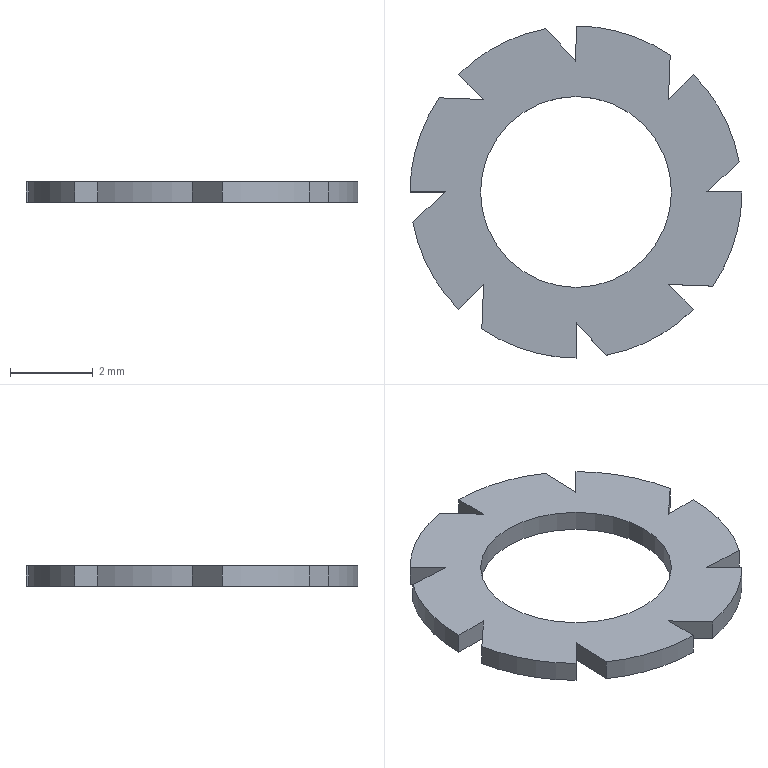Part | NX | features BREP 1 | 1 solid | 27 faces | box 8 x 8 x 0.5 mm | volume 15.56 mm3 | plane 18 | cylinder 9 | commonest cylinder face diameters 8 x8 4.6 x1
STEP:
#1=CARTESIAN_POINT('',(2.3,0.,0.));
#2=VERTEX_POINT('',#1);
#3=CARTESIAN_POINT('',(0.,0.,0.));
#4=DIRECTION('',(0.,0.,1.));
#5=DIRECTION('',(1.,0.,0.));
#6=AXIS2_PLACEMENT_3D('',#3,#4,#5);
#7=CIRCLE('',#6,2.3);
#8=EDGE_CURVE('',#2,#2,#7,.T.);
#9=ORIENTED_EDGE('',*,*,#8,.T.);
#10=EDGE_LOOP('',(#9));
#11=FACE_BOUND('',#10,.T.);
#12=CARTESIAN_POINT('',(2.3,0.,-0.5));
#13=VERTEX_POINT('',#12);
#14=CARTESIAN_POINT('',(0.,0.,-0.5));
#15=DIRECTION('',(0.,0.,1.));
#16=DIRECTION('',(1.,0.,0.));
#17=AXIS2_PLACEMENT_3D('',#14,#15,#16);
#18=CIRCLE('',#17,2.3);
#19=EDGE_CURVE('',#13,#13,#18,.T.);
#20=ORIENTED_EDGE('',*,*,#19,.F.);
#21=EDGE_LOOP('',(#20));
#22=FACE_BOUND('',#21,.T.);
#23=CARTESIAN_POINT('',(0.,0.,-0.5));
#24=DIRECTION('',(0.,0.,1.));
#25=DIRECTION('',(1.,0.,0.));
#26=AXIS2_PLACEMENT_3D('',#23,#24,#25);
#27=CYLINDRICAL_SURFACE('',#26,2.3);
#28=ADVANCED_FACE('',(#11,#22),#27,.F.);
#29=CARTESIAN_POINT('',(2.828,2.828,-0.5));
#30=VERTEX_POINT('',#29);
#31=CARTESIAN_POINT('',(2.828,2.828,0.));
#32=VERTEX_POINT('',#31);
#33=CARTESIAN_POINT('',(2.828,2.828,-0.5));
#34=DIRECTION('',(0.,0.,1.));
#35=VECTOR('',#34,1000.);
#36=LINE('',#33,#35);
#37=EDGE_CURVE('',#30,#32,#36,.T.);
#38=ORIENTED_EDGE('',*,*,#37,.T.);
#39=CARTESIAN_POINT('',(3.934,0.7243,0.));
#40=VERTEX_POINT('',#39);
#41=CARTESIAN_POINT('',(0.,0.,0.));
#42=DIRECTION('',(0.,0.,1.));
#43=DIRECTION('',(1.,0.,0.));
#44=AXIS2_PLACEMENT_3D('',#41,#42,#43);
#45=CIRCLE('',#44,4.);
#46=EDGE_CURVE('',#40,#32,#45,.T.);
#47=ORIENTED_EDGE('',*,*,#46,.F.);
#48=CARTESIAN_POINT('',(3.934,0.7243,-0.5));
#49=VERTEX_POINT('',#48);
#50=CARTESIAN_POINT('',(3.934,0.7243,-0.5));
#51=DIRECTION('',(0.,0.,1.));
#52=VECTOR('',#51,1000.);
#53=LINE('',#50,#52);
#54=EDGE_CURVE('',#49,#40,#53,.T.);
#55=ORIENTED_EDGE('',*,*,#54,.F.);
#56=CARTESIAN_POINT('',(0.,0.,-0.5));
#57=DIRECTION('',(0.,0.,1.));
#58=DIRECTION('',(1.,0.,0.));
#59=AXIS2_PLACEMENT_3D('',#56,#57,#58);
#60=CIRCLE('',#59,4.);
#61=EDGE_CURVE('',#49,#30,#60,.T.);
#62=ORIENTED_EDGE('',*,*,#61,.T.);
#63=EDGE_LOOP('',(#38,#47,#55,#62));
#64=FACE_BOUND('',#63,.T.);
#65=CARTESIAN_POINT('',(0.,0.,-0.5));
#66=DIRECTION('',(0.,0.,1.));
#67=DIRECTION('',(1.,0.,0.));
#68=AXIS2_PLACEMENT_3D('',#65,#66,#67);
#69=CYLINDRICAL_SURFACE('',#68,4.);
#70=ADVANCED_FACE('',(#64),#69,.T.);
#71=CARTESIAN_POINT('',(4.,0.,-0.5));
#72=VERTEX_POINT('',#71);
#73=CARTESIAN_POINT('',(4.,0.,0.));
#74=VERTEX_POINT('',#73);
#75=CARTESIAN_POINT('',(4.,0.,-0.5));
#76=DIRECTION('',(0.,0.,1.));
#77=VECTOR('',#76,1000.);
#78=LINE('',#75,#77);
#79=EDGE_CURVE('',#72,#74,#78,.T.);
#80=ORIENTED_EDGE('',*,*,#79,.T.);
#81=CARTESIAN_POINT('',(3.294,-2.27,0.));
#82=VERTEX_POINT('',#81);
#83=CARTESIAN_POINT('',(0.,0.,0.));
#84=DIRECTION('',(0.,0.,1.));
#85=DIRECTION('',(1.,0.,0.));
#86=AXIS2_PLACEMENT_3D('',#83,#84,#85);
#87=CIRCLE('',#86,4.);
#88=EDGE_CURVE('',#82,#74,#87,.T.);
#89=ORIENTED_EDGE('',*,*,#88,.F.);
#90=CARTESIAN_POINT('',(3.294,-2.27,-0.5));
#91=VERTEX_POINT('',#90);
#92=CARTESIAN_POINT('',(3.294,-2.27,-0.5));
#93=DIRECTION('',(0.,0.,1.));
#94=VECTOR('',#93,1000.);
#95=LINE('',#92,#94);
#96=EDGE_CURVE('',#91,#82,#95,.T.);
#97=ORIENTED_EDGE('',*,*,#96,.F.);
#98=CARTESIAN_POINT('',(0.,0.,-0.5));
#99=DIRECTION('',(0.,0.,1.));
#100=DIRECTION('',(1.,0.,0.));
#101=AXIS2_PLACEMENT_3D('',#98,#99,#100);
#102=CIRCLE('',#101,4.);
#103=EDGE_CURVE('',#91,#72,#102,.T.);
#104=ORIENTED_EDGE('',*,*,#103,.T.);
#105=EDGE_LOOP('',(#80,#89,#97,#104));
#106=FACE_BOUND('',#105,.T.);
#107=CARTESIAN_POINT('',(0.,0.,-0.5));
#108=DIRECTION('',(0.,0.,1.));
#109=DIRECTION('',(1.,0.,0.));
#110=AXIS2_PLACEMENT_3D('',#107,#108,#109);
#111=CYLINDRICAL_SURFACE('',#110,4.);
#112=ADVANCED_FACE('',(#106),#111,.T.);
#113=CARTESIAN_POINT('',(2.828,-2.828,-0.5));
#114=VERTEX_POINT('',#113);
#115=CARTESIAN_POINT('',(2.828,-2.828,0.));
#116=VERTEX_POINT('',#115);
#117=CARTESIAN_POINT('',(2.828,-2.828,-0.5));
#118=DIRECTION('',(0.,0.,1.));
#119=VECTOR('',#118,1000.);
#120=LINE('',#117,#119);
#121=EDGE_CURVE('',#114,#116,#120,.T.);
#122=ORIENTED_EDGE('',*,*,#121,.T.);
#123=CARTESIAN_POINT('',(0.7243,-3.934,0.));
#124=VERTEX_POINT('',#123);
#125=CARTESIAN_POINT('',(0.,0.,0.));
#126=DIRECTION('',(0.,0.,1.));
#127=DIRECTION('',(1.,0.,0.));
#128=AXIS2_PLACEMENT_3D('',#125,#126,#127);
#129=CIRCLE('',#128,4.);
#130=EDGE_CURVE('',#124,#116,#129,.T.);
#131=ORIENTED_EDGE('',*,*,#130,.F.);
#132=CARTESIAN_POINT('',(0.7243,-3.934,-0.5));
#133=VERTEX_POINT('',#132);
#134=CARTESIAN_POINT('',(0.7243,-3.934,-0.5));
#135=DIRECTION('',(0.,0.,1.));
#136=VECTOR('',#135,1000.);
#137=LINE('',#134,#136);
#138=EDGE_CURVE('',#133,#124,#137,.T.);
#139=ORIENTED_EDGE('',*,*,#138,.F.);
#140=CARTESIAN_POINT('',(0.,0.,-0.5));
#141=DIRECTION('',(0.,0.,1.));
#142=DIRECTION('',(1.,0.,0.));
#143=AXIS2_PLACEMENT_3D('',#140,#141,#142);
#144=CIRCLE('',#143,4.);
#145=EDGE_CURVE('',#133,#114,#144,.T.);
#146=ORIENTED_EDGE('',*,*,#145,.T.);
#147=EDGE_LOOP('',(#122,#131,#139,#146));
#148=FACE_BOUND('',#147,.T.);
#149=CARTESIAN_POINT('',(0.,0.,-0.5));
#150=DIRECTION('',(0.,0.,1.));
#151=DIRECTION('',(1.,0.,0.));
#152=AXIS2_PLACEMENT_3D('',#149,#150,#151);
#153=CYLINDRICAL_SURFACE('',#152,4.);
#154=ADVANCED_FACE('',(#148),#153,.T.);
#155=CARTESIAN_POINT('',(0.,-4.,-0.5));
#156=VERTEX_POINT('',#155);
#157=CARTESIAN_POINT('',(0.,-4.,0.));
#158=VERTEX_POINT('',#157);
#159=CARTESIAN_POINT('',(0.,-4.,-0.5));
#160=DIRECTION('',(0.,0.,1.));
#161=VECTOR('',#160,1000.);
#162=LINE('',#159,#161);
#163=EDGE_CURVE('',#156,#158,#162,.T.);
#164=ORIENTED_EDGE('',*,*,#163,.T.);
#165=CARTESIAN_POINT('',(-2.27,-3.294,0.));
#166=VERTEX_POINT('',#165);
#167=CARTESIAN_POINT('',(0.,0.,0.));
#168=DIRECTION('',(0.,0.,1.));
#169=DIRECTION('',(1.,0.,0.));
#170=AXIS2_PLACEMENT_3D('',#167,#168,#169);
#171=CIRCLE('',#170,4.);
#172=EDGE_CURVE('',#166,#158,#171,.T.);
#173=ORIENTED_EDGE('',*,*,#172,.F.);
#174=CARTESIAN_POINT('',(-2.27,-3.294,-0.5));
#175=VERTEX_POINT('',#174);
#176=CARTESIAN_POINT('',(-2.27,-3.294,-0.5));
#177=DIRECTION('',(0.,0.,1.));
#178=VECTOR('',#177,1000.);
#179=LINE('',#176,#178);
#180=EDGE_CURVE('',#175,#166,#179,.T.);
#181=ORIENTED_EDGE('',*,*,#180,.F.);
#182=CARTESIAN_POINT('',(0.,0.,-0.5));
#183=DIRECTION('',(0.,0.,1.));
#184=DIRECTION('',(1.,0.,0.));
#185=AXIS2_PLACEMENT_3D('',#182,#183,#184);
#186=CIRCLE('',#185,4.);
#187=EDGE_CURVE('',#175,#156,#186,.T.);
#188=ORIENTED_EDGE('',*,*,#187,.T.);
#189=EDGE_LOOP('',(#164,#173,#181,#188));
#190=FACE_BOUND('',#189,.T.);
#191=CARTESIAN_POINT('',(0.,0.,-0.5));
#192=DIRECTION('',(0.,0.,1.));
#193=DIRECTION('',(1.,0.,0.));
#194=AXIS2_PLACEMENT_3D('',#191,#192,#193);
#195=CYLINDRICAL_SURFACE('',#194,4.);
#196=ADVANCED_FACE('',(#190),#195,.T.);
#197=CARTESIAN_POINT('',(-2.828,-2.828,-0.5));
#198=VERTEX_POINT('',#197);
#199=CARTESIAN_POINT('',(-2.828,-2.828,0.));
#200=VERTEX_POINT('',#199);
#201=CARTESIAN_POINT('',(-2.828,-2.828,-0.5));
#202=DIRECTION('',(0.,0.,1.));
#203=VECTOR('',#202,1000.);
#204=LINE('',#201,#203);
#205=EDGE_CURVE('',#198,#200,#204,.T.);
#206=ORIENTED_EDGE('',*,*,#205,.T.);
#207=CARTESIAN_POINT('',(-3.934,-0.7243,0.));
#208=VERTEX_POINT('',#207);
#209=CARTESIAN_POINT('',(0.,0.,0.));
#210=DIRECTION('',(0.,0.,1.));
#211=DIRECTION('',(1.,0.,0.));
#212=AXIS2_PLACEMENT_3D('',#209,#210,#211);
#213=CIRCLE('',#212,4.);
#214=EDGE_CURVE('',#208,#200,#213,.T.);
#215=ORIENTED_EDGE('',*,*,#214,.F.);
#216=CARTESIAN_POINT('',(-3.934,-0.7243,-0.5));
#217=VERTEX_POINT('',#216);
#218=CARTESIAN_POINT('',(-3.934,-0.7243,-0.5));
#219=DIRECTION('',(0.,0.,1.));
#220=VECTOR('',#219,1000.);
#221=LINE('',#218,#220);
#222=EDGE_CURVE('',#217,#208,#221,.T.);
#223=ORIENTED_EDGE('',*,*,#222,.F.);
#224=CARTESIAN_POINT('',(0.,0.,-0.5));
#225=DIRECTION('',(0.,0.,1.));
#226=DIRECTION('',(1.,0.,0.));
#227=AXIS2_PLACEMENT_3D('',#224,#225,#226);
#228=CIRCLE('',#227,4.);
#229=EDGE_CURVE('',#217,#198,#228,.T.);
#230=ORIENTED_EDGE('',*,*,#229,.T.);
#231=EDGE_LOOP('',(#206,#215,#223,#230));
#232=FACE_BOUND('',#231,.T.);
#233=CARTESIAN_POINT('',(0.,0.,-0.5));
#234=DIRECTION('',(0.,0.,1.));
#235=DIRECTION('',(1.,0.,0.));
#236=AXIS2_PLACEMENT_3D('',#233,#234,#235);
#237=CYLINDRICAL_SURFACE('',#236,4.);
#238=ADVANCED_FACE('',(#232),#237,.T.);
#239=CARTESIAN_POINT('',(-4.,0.,-0.5));
#240=VERTEX_POINT('',#239);
#241=CARTESIAN_POINT('',(-4.,0.,0.));
#242=VERTEX_POINT('',#241);
#243=CARTESIAN_POINT('',(-4.,0.,-0.5));
#244=DIRECTION('',(0.,0.,1.));
#245=VECTOR('',#244,1000.);
#246=LINE('',#243,#245);
#247=EDGE_CURVE('',#240,#242,#246,.T.);
#248=ORIENTED_EDGE('',*,*,#247,.T.);
#249=CARTESIAN_POINT('',(-3.294,2.27,0.));
#250=VERTEX_POINT('',#249);
#251=CARTESIAN_POINT('',(0.,0.,0.));
#252=DIRECTION('',(0.,0.,1.));
#253=DIRECTION('',(1.,0.,0.));
#254=AXIS2_PLACEMENT_3D('',#251,#252,#253);
#255=CIRCLE('',#254,4.);
#256=EDGE_CURVE('',#250,#242,#255,.T.);
#257=ORIENTED_EDGE('',*,*,#256,.F.);
#258=CARTESIAN_POINT('',(-3.294,2.27,-0.5));
#259=VERTEX_POINT('',#258);
#260=CARTESIAN_POINT('',(-3.294,2.27,-0.5));
#261=DIRECTION('',(0.,0.,1.));
#262=VECTOR('',#261,1000.);
#263=LINE('',#260,#262);
#264=EDGE_CURVE('',#259,#250,#263,.T.);
#265=ORIENTED_EDGE('',*,*,#264,.F.);
#266=CARTESIAN_POINT('',(0.,0.,-0.5));
#267=DIRECTION('',(0.,0.,1.));
#268=DIRECTION('',(1.,0.,0.));
#269=AXIS2_PLACEMENT_3D('',#266,#267,#268);
#270=CIRCLE('',#269,4.);
#271=EDGE_CURVE('',#259,#240,#270,.T.);
#272=ORIENTED_EDGE('',*,*,#271,.T.);
#273=EDGE_LOOP('',(#248,#257,#265,#272));
#274=FACE_BOUND('',#273,.T.);
#275=CARTESIAN_POINT('',(0.,0.,-0.5));
#276=DIRECTION('',(0.,0.,1.));
#277=DIRECTION('',(1.,0.,0.));
#278=AXIS2_PLACEMENT_3D('',#275,#276,#277);
#279=CYLINDRICAL_SURFACE('',#278,4.);
#280=ADVANCED_FACE('',(#274),#279,.T.);
#281=CARTESIAN_POINT('',(-2.828,2.828,-0.5));
#282=VERTEX_POINT('',#281);
#283=CARTESIAN_POINT('',(-2.828,2.828,0.));
#284=VERTEX_POINT('',#283);
#285=CARTESIAN_POINT('',(-2.828,2.828,-0.5));
#286=DIRECTION('',(0.,0.,1.));
#287=VECTOR('',#286,1000.);
#288=LINE('',#285,#287);
#289=EDGE_CURVE('',#282,#284,#288,.T.);
#290=ORIENTED_EDGE('',*,*,#289,.T.);
#291=CARTESIAN_POINT('',(-0.7243,3.934,0.));
#292=VERTEX_POINT('',#291);
#293=CARTESIAN_POINT('',(0.,0.,0.));
#294=DIRECTION('',(0.,0.,1.));
#295=DIRECTION('',(1.,0.,0.));
#296=AXIS2_PLACEMENT_3D('',#293,#294,#295);
#297=CIRCLE('',#296,4.);
#298=EDGE_CURVE('',#292,#284,#297,.T.);
#299=ORIENTED_EDGE('',*,*,#298,.F.);
#300=CARTESIAN_POINT('',(-0.7243,3.934,-0.5));
#301=VERTEX_POINT('',#300);
#302=CARTESIAN_POINT('',(-0.7243,3.934,-0.5));
#303=DIRECTION('',(0.,0.,1.));
#304=VECTOR('',#303,1000.);
#305=LINE('',#302,#304);
#306=EDGE_CURVE('',#301,#292,#305,.T.);
#307=ORIENTED_EDGE('',*,*,#306,.F.);
#308=CARTESIAN_POINT('',(0.,0.,-0.5));
#309=DIRECTION('',(0.,0.,1.));
#310=DIRECTION('',(1.,0.,0.));
#311=AXIS2_PLACEMENT_3D('',#308,#309,#310);
#312=CIRCLE('',#311,4.);
#313=EDGE_CURVE('',#301,#282,#312,.T.);
#314=ORIENTED_EDGE('',*,*,#313,.T.);
#315=EDGE_LOOP('',(#290,#299,#307,#314));
#316=FACE_BOUND('',#315,.T.);
#317=CARTESIAN_POINT('',(0.,0.,-0.5));
#318=DIRECTION('',(0.,0.,1.));
#319=DIRECTION('',(1.,0.,0.));
#320=AXIS2_PLACEMENT_3D('',#317,#318,#319);
#321=CYLINDRICAL_SURFACE('',#320,4.);
#322=ADVANCED_FACE('',(#316),#321,.T.);
#323=CARTESIAN_POINT('',(2.27,3.294,-0.5));
#324=VERTEX_POINT('',#323);
#325=CARTESIAN_POINT('',(2.27,3.294,0.));
#326=VERTEX_POINT('',#325);
#327=CARTESIAN_POINT('',(2.27,3.294,-0.5));
#328=DIRECTION('',(0.,0.,1.));
#329=VECTOR('',#328,1000.);
#330=LINE('',#327,#329);
#331=EDGE_CURVE('',#324,#326,#330,.T.);
#332=ORIENTED_EDGE('',*,*,#331,.F.);
#333=CARTESIAN_POINT('',(0.,4.,-0.5));
#334=VERTEX_POINT('',#333);
#335=CARTESIAN_POINT('',(0.,0.,-0.5));
#336=DIRECTION('',(0.,0.,1.));
#337=DIRECTION('',(1.,0.,0.));
#338=AXIS2_PLACEMENT_3D('',#335,#336,#337);
#339=CIRCLE('',#338,4.);
#340=EDGE_CURVE('',#324,#334,#339,.T.);
#341=ORIENTED_EDGE('',*,*,#340,.T.);
#342=CARTESIAN_POINT('',(0.,4.,0.));
#343=VERTEX_POINT('',#342);
#344=CARTESIAN_POINT('',(0.,4.,-0.5));
#345=DIRECTION('',(0.,0.,1.));
#346=VECTOR('',#345,1000.);
#347=LINE('',#344,#346);
#348=EDGE_CURVE('',#334,#343,#347,.T.);
#349=ORIENTED_EDGE('',*,*,#348,.T.);
#350=CARTESIAN_POINT('',(0.,0.,0.));
#351=DIRECTION('',(0.,0.,1.));
#352=DIRECTION('',(1.,0.,0.));
#353=AXIS2_PLACEMENT_3D('',#350,#351,#352);
#354=CIRCLE('',#353,4.);
#355=EDGE_CURVE('',#326,#343,#354,.T.);
#356=ORIENTED_EDGE('',*,*,#355,.F.);
#357=EDGE_LOOP('',(#332,#341,#349,#356));
#358=FACE_BOUND('',#357,.T.);
#359=CARTESIAN_POINT('',(0.,0.,-0.5));
#360=DIRECTION('',(0.,0.,1.));
#361=DIRECTION('',(1.,0.,0.));
#362=AXIS2_PLACEMENT_3D('',#359,#360,#361);
#363=CYLINDRICAL_SURFACE('',#362,4.);
#364=ADVANCED_FACE('',(#358),#363,.T.);
#365=ORIENTED_EDGE('',*,*,#19,.T.);
#366=EDGE_LOOP('',(#365));
#367=FACE_BOUND('',#366,.T.);
#368=CARTESIAN_POINT('',(2.227,2.227,-0.5));
#369=VERTEX_POINT('',#368);
#370=CARTESIAN_POINT('',(2.227,2.227,-0.5));
#371=DIRECTION('',(-0.03947,-0.9992,0.));
#372=VECTOR('',#371,1000.);
#373=LINE('',#370,#372);
#374=EDGE_CURVE('',#324,#369,#373,.T.);
#375=ORIENTED_EDGE('',*,*,#374,.T.);
#376=CARTESIAN_POINT('',(2.828,2.828,-0.5));
#377=DIRECTION('',(0.7071,0.7071,0.));
#378=VECTOR('',#377,1000.);
#379=LINE('',#376,#378);
#380=EDGE_CURVE('',#369,#30,#379,.T.);
#381=ORIENTED_EDGE('',*,*,#380,.T.);
#382=ORIENTED_EDGE('',*,*,#61,.F.);
#383=CARTESIAN_POINT('',(3.15,0.,-0.5));
#384=VERTEX_POINT('',#383);
#385=CARTESIAN_POINT('',(3.15,0.,-0.5));
#386=DIRECTION('',(-0.7345,-0.6786,0.));
#387=VECTOR('',#386,1000.);
#388=LINE('',#385,#387);
#389=EDGE_CURVE('',#49,#384,#388,.T.);
#390=ORIENTED_EDGE('',*,*,#389,.T.);
#391=CARTESIAN_POINT('',(4.,0.,-0.5));
#392=DIRECTION('',(1.,0.,0.));
#393=VECTOR('',#392,1000.);
#394=LINE('',#391,#393);
#395=EDGE_CURVE('',#384,#72,#394,.T.);
#396=ORIENTED_EDGE('',*,*,#395,.T.);
#397=ORIENTED_EDGE('',*,*,#103,.F.);
#398=CARTESIAN_POINT('',(2.227,-2.227,-0.5));
#399=VERTEX_POINT('',#398);
#400=CARTESIAN_POINT('',(2.227,-2.227,-0.5));
#401=DIRECTION('',(-0.9992,0.03947,0.));
#402=VECTOR('',#401,1000.);
#403=LINE('',#400,#402);
#404=EDGE_CURVE('',#91,#399,#403,.T.);
#405=ORIENTED_EDGE('',*,*,#404,.T.);
#406=CARTESIAN_POINT('',(2.828,-2.828,-0.5));
#407=DIRECTION('',(0.7071,-0.7071,0.));
#408=VECTOR('',#407,1000.);
#409=LINE('',#406,#408);
#410=EDGE_CURVE('',#399,#114,#409,.T.);
#411=ORIENTED_EDGE('',*,*,#410,.T.);
#412=ORIENTED_EDGE('',*,*,#145,.F.);
#413=CARTESIAN_POINT('',(0.,-3.15,-0.5));
#414=VERTEX_POINT('',#413);
#415=CARTESIAN_POINT('',(0.,-3.15,-0.5));
#416=DIRECTION('',(-0.6786,0.7345,0.));
#417=VECTOR('',#416,1000.);
#418=LINE('',#415,#417);
#419=EDGE_CURVE('',#133,#414,#418,.T.);
#420=ORIENTED_EDGE('',*,*,#419,.T.);
#421=CARTESIAN_POINT('',(0.,-4.,-0.5));
#422=DIRECTION('',(0.,-1.,0.));
#423=VECTOR('',#422,1000.);
#424=LINE('',#421,#423);
#425=EDGE_CURVE('',#414,#156,#424,.T.);
#426=ORIENTED_EDGE('',*,*,#425,.T.);
#427=ORIENTED_EDGE('',*,*,#187,.F.);
#428=CARTESIAN_POINT('',(-2.227,-2.227,-0.5));
#429=VERTEX_POINT('',#428);
#430=CARTESIAN_POINT('',(-2.227,-2.227,-0.5));
#431=DIRECTION('',(0.03947,0.9992,0.));
#432=VECTOR('',#431,1000.);
#433=LINE('',#430,#432);
#434=EDGE_CURVE('',#175,#429,#433,.T.);
#435=ORIENTED_EDGE('',*,*,#434,.T.);
#436=CARTESIAN_POINT('',(-2.828,-2.828,-0.5));
#437=DIRECTION('',(-0.7071,-0.7071,0.));
#438=VECTOR('',#437,1000.);
#439=LINE('',#436,#438);
#440=EDGE_CURVE('',#429,#198,#439,.T.);
#441=ORIENTED_EDGE('',*,*,#440,.T.);
#442=ORIENTED_EDGE('',*,*,#229,.F.);
#443=CARTESIAN_POINT('',(-3.15,0.,-0.5));
#444=VERTEX_POINT('',#443);
#445=CARTESIAN_POINT('',(-3.15,0.,-0.5));
#446=DIRECTION('',(0.7345,0.6786,0.));
#447=VECTOR('',#446,1000.);
#448=LINE('',#445,#447);
#449=EDGE_CURVE('',#217,#444,#448,.T.);
#450=ORIENTED_EDGE('',*,*,#449,.T.);
#451=CARTESIAN_POINT('',(-4.,0.,-0.5));
#452=DIRECTION('',(-1.,0.,0.));
#453=VECTOR('',#452,1000.);
#454=LINE('',#451,#453);
#455=EDGE_CURVE('',#444,#240,#454,.T.);
#456=ORIENTED_EDGE('',*,*,#455,.T.);
#457=ORIENTED_EDGE('',*,*,#271,.F.);
#458=CARTESIAN_POINT('',(-2.227,2.227,-0.5));
#459=VERTEX_POINT('',#458);
#460=CARTESIAN_POINT('',(-2.227,2.227,-0.5));
#461=DIRECTION('',(0.9992,-0.03947,0.));
#462=VECTOR('',#461,1000.);
#463=LINE('',#460,#462);
#464=EDGE_CURVE('',#259,#459,#463,.T.);
#465=ORIENTED_EDGE('',*,*,#464,.T.);
#466=CARTESIAN_POINT('',(-2.828,2.828,-0.5));
#467=DIRECTION('',(-0.7071,0.7071,0.));
#468=VECTOR('',#467,1000.);
#469=LINE('',#466,#468);
#470=EDGE_CURVE('',#459,#282,#469,.T.);
#471=ORIENTED_EDGE('',*,*,#470,.T.);
#472=ORIENTED_EDGE('',*,*,#313,.F.);
#473=CARTESIAN_POINT('',(0.,3.15,-0.5));
#474=VERTEX_POINT('',#473);
#475=CARTESIAN_POINT('',(0.,3.15,-0.5));
#476=DIRECTION('',(0.6786,-0.7345,0.));
#477=VECTOR('',#476,1000.);
#478=LINE('',#475,#477);
#479=EDGE_CURVE('',#301,#474,#478,.T.);
#480=ORIENTED_EDGE('',*,*,#479,.T.);
#481=CARTESIAN_POINT('',(0.,4.,-0.5));
#482=DIRECTION('',(0.,1.,0.));
#483=VECTOR('',#482,1000.);
#484=LINE('',#481,#483);
#485=EDGE_CURVE('',#474,#334,#484,.T.);
#486=ORIENTED_EDGE('',*,*,#485,.T.);
#487=ORIENTED_EDGE('',*,*,#340,.F.);
#488=EDGE_LOOP('',(#375,#381,#382,#390,#396,#397,#405,#411,#412,#420,#426,#427,#435,#441,#442,#450,#456,#457,#465,#471,#472,#480,#486,#487));
#489=FACE_BOUND('',#488,.T.);
#490=CARTESIAN_POINT('',(0.,0.,-0.5));
#491=DIRECTION('',(0.,0.,1.));
#492=DIRECTION('',(1.,0.,0.));
#493=AXIS2_PLACEMENT_3D('',#490,#491,#492);
#494=PLANE('',#493);
#495=ADVANCED_FACE('',(#367,#489),#494,.F.);
#496=CARTESIAN_POINT('',(2.227,2.227,0.));
#497=VERTEX_POINT('',#496);
#498=CARTESIAN_POINT('',(2.828,2.828,0.));
#499=DIRECTION('',(0.7071,0.7071,0.));
#500=VECTOR('',#499,1000.);
#501=LINE('',#498,#500);
#502=EDGE_CURVE('',#497,#32,#501,.T.);
#503=ORIENTED_EDGE('',*,*,#502,.F.);
#504=CARTESIAN_POINT('',(2.136,-0.08438,0.));
#505=DIRECTION('',(-0.03947,-0.9992,0.));
#506=VECTOR('',#505,1000.);
#507=LINE('',#504,#506);
#508=EDGE_CURVE('',#326,#497,#507,.T.);
#509=ORIENTED_EDGE('',*,*,#508,.F.);
#510=ORIENTED_EDGE('',*,*,#355,.T.);
#511=CARTESIAN_POINT('',(0.,3.15,0.));
#512=VERTEX_POINT('',#511);
#513=CARTESIAN_POINT('',(0.,4.,0.));
#514=DIRECTION('',(0.,1.,0.));
#515=VECTOR('',#514,1000.);
#516=LINE('',#513,#515);
#517=EDGE_CURVE('',#512,#343,#516,.T.);
#518=ORIENTED_EDGE('',*,*,#517,.F.);
#519=CARTESIAN_POINT('',(1.57,1.451,0.));
#520=DIRECTION('',(0.6786,-0.7345,0.));
#521=VECTOR('',#520,1000.);
#522=LINE('',#519,#521);
#523=EDGE_CURVE('',#292,#512,#522,.T.);
#524=ORIENTED_EDGE('',*,*,#523,.F.);
#525=ORIENTED_EDGE('',*,*,#298,.T.);
#526=CARTESIAN_POINT('',(-2.227,2.227,0.));
#527=VERTEX_POINT('',#526);
#528=CARTESIAN_POINT('',(-2.828,2.828,0.));
#529=DIRECTION('',(-0.7071,0.7071,0.));
#530=VECTOR('',#529,1000.);
#531=LINE('',#528,#530);
#532=EDGE_CURVE('',#527,#284,#531,.T.);
#533=ORIENTED_EDGE('',*,*,#532,.F.);
#534=CARTESIAN_POINT('',(0.08438,2.136,0.));
#535=DIRECTION('',(0.9992,-0.03947,0.));
#536=VECTOR('',#535,1000.);
#537=LINE('',#534,#536);
#538=EDGE_CURVE('',#250,#527,#537,.T.);
#539=ORIENTED_EDGE('',*,*,#538,.F.);
#540=ORIENTED_EDGE('',*,*,#256,.T.);
#541=CARTESIAN_POINT('',(-3.15,0.,0.));
#542=VERTEX_POINT('',#541);
#543=CARTESIAN_POINT('',(-4.,0.,0.));
#544=DIRECTION('',(-1.,0.,0.));
#545=VECTOR('',#544,1000.);
#546=LINE('',#543,#545);
#547=EDGE_CURVE('',#542,#242,#546,.T.);
#548=ORIENTED_EDGE('',*,*,#547,.F.);
#549=CARTESIAN_POINT('',(-1.451,1.57,0.));
#550=DIRECTION('',(0.7345,0.6786,0.));
#551=VECTOR('',#550,1000.);
#552=LINE('',#549,#551);
#553=EDGE_CURVE('',#208,#542,#552,.T.);
#554=ORIENTED_EDGE('',*,*,#553,.F.);
#555=ORIENTED_EDGE('',*,*,#214,.T.);
#556=CARTESIAN_POINT('',(-2.227,-2.227,0.));
#557=VERTEX_POINT('',#556);
#558=CARTESIAN_POINT('',(-2.828,-2.828,0.));
#559=DIRECTION('',(-0.7071,-0.7071,0.));
#560=VECTOR('',#559,1000.);
#561=LINE('',#558,#560);
#562=EDGE_CURVE('',#557,#200,#561,.T.);
#563=ORIENTED_EDGE('',*,*,#562,.F.);
#564=CARTESIAN_POINT('',(-2.136,0.08438,0.));
#565=DIRECTION('',(0.03947,0.9992,0.));
#566=VECTOR('',#565,1000.);
#567=LINE('',#564,#566);
#568=EDGE_CURVE('',#166,#557,#567,.T.);
#569=ORIENTED_EDGE('',*,*,#568,.F.);
#570=ORIENTED_EDGE('',*,*,#172,.T.);
#571=CARTESIAN_POINT('',(0.,-3.15,0.));
#572=VERTEX_POINT('',#571);
#573=CARTESIAN_POINT('',(0.,-4.,0.));
#574=DIRECTION('',(0.,-1.,0.));
#575=VECTOR('',#574,1000.);
#576=LINE('',#573,#575);
#577=EDGE_CURVE('',#572,#158,#576,.T.);
#578=ORIENTED_EDGE('',*,*,#577,.F.);
#579=CARTESIAN_POINT('',(-1.57,-1.451,0.));
#580=DIRECTION('',(-0.6786,0.7345,0.));
#581=VECTOR('',#580,1000.);
#582=LINE('',#579,#581);
#583=EDGE_CURVE('',#124,#572,#582,.T.);
#584=ORIENTED_EDGE('',*,*,#583,.F.);
#585=ORIENTED_EDGE('',*,*,#130,.T.);
#586=CARTESIAN_POINT('',(2.227,-2.227,0.));
#587=VERTEX_POINT('',#586);
#588=CARTESIAN_POINT('',(2.828,-2.828,0.));
#589=DIRECTION('',(0.7071,-0.7071,0.));
#590=VECTOR('',#589,1000.);
#591=LINE('',#588,#590);
#592=EDGE_CURVE('',#587,#116,#591,.T.);
#593=ORIENTED_EDGE('',*,*,#592,.F.);
#594=CARTESIAN_POINT('',(-0.08438,-2.136,0.));
#595=DIRECTION('',(-0.9992,0.03947,0.));
#596=VECTOR('',#595,1000.);
#597=LINE('',#594,#596);
#598=EDGE_CURVE('',#82,#587,#597,.T.);
#599=ORIENTED_EDGE('',*,*,#598,.F.);
#600=ORIENTED_EDGE('',*,*,#88,.T.);
#601=CARTESIAN_POINT('',(3.15,0.,0.));
#602=VERTEX_POINT('',#601);
#603=CARTESIAN_POINT('',(4.,0.,0.));
#604=DIRECTION('',(1.,0.,0.));
#605=VECTOR('',#604,1000.);
#606=LINE('',#603,#605);
#607=EDGE_CURVE('',#602,#74,#606,.T.);
#608=ORIENTED_EDGE('',*,*,#607,.F.);
#609=CARTESIAN_POINT('',(1.451,-1.57,0.));
#610=DIRECTION('',(-0.7345,-0.6786,0.));
#611=VECTOR('',#610,1000.);
#612=LINE('',#609,#611);
#613=EDGE_CURVE('',#40,#602,#612,.T.);
#614=ORIENTED_EDGE('',*,*,#613,.F.);
#615=ORIENTED_EDGE('',*,*,#46,.T.);
#616=EDGE_LOOP('',(#503,#509,#510,#518,#524,#525,#533,#539,#540,#548,#554,#555,#563,#569,#570,#578,#584,#585,#593,#599,#600,#608,#614,#615));
#617=FACE_BOUND('',#616,.T.);
#618=ORIENTED_EDGE('',*,*,#8,.F.);
#619=EDGE_LOOP('',(#618));
#620=FACE_BOUND('',#619,.T.);
#621=CARTESIAN_POINT('',(0.,0.,0.));
#622=DIRECTION('',(0.,0.,1.));
#623=DIRECTION('',(1.,0.,0.));
#624=AXIS2_PLACEMENT_3D('',#621,#622,#623);
#625=PLANE('',#624);
#626=ADVANCED_FACE('',(#617,#620),#625,.T.);
#627=ORIENTED_EDGE('',*,*,#517,.T.);
#628=ORIENTED_EDGE('',*,*,#348,.F.);
#629=ORIENTED_EDGE('',*,*,#485,.F.);
#630=CARTESIAN_POINT('',(0.,3.15,-0.5));
#631=DIRECTION('',(0.,0.,1.));
#632=VECTOR('',#631,1000.);
#633=LINE('',#630,#632);
#634=EDGE_CURVE('',#474,#512,#633,.T.);
#635=ORIENTED_EDGE('',*,*,#634,.T.);
#636=EDGE_LOOP('',(#627,#628,#629,#635));
#637=FACE_BOUND('',#636,.T.);
#638=CARTESIAN_POINT('',(0.,4.,-0.5));
#639=DIRECTION('',(1.,0.,0.));
#640=DIRECTION('',(0.,1.,0.));
#641=AXIS2_PLACEMENT_3D('',#638,#639,#640);
#642=PLANE('',#641);
#643=ADVANCED_FACE('',(#637),#642,.F.);
#644=ORIENTED_EDGE('',*,*,#306,.T.);
#645=ORIENTED_EDGE('',*,*,#523,.T.);
#646=ORIENTED_EDGE('',*,*,#634,.F.);
#647=ORIENTED_EDGE('',*,*,#479,.F.);
#648=EDGE_LOOP('',(#644,#645,#646,#647));
#649=FACE_BOUND('',#648,.T.);
#650=CARTESIAN_POINT('',(0.,3.15,-0.5));
#651=DIRECTION('',(-0.7345,-0.6786,0.));
#652=DIRECTION('',(0.6786,-0.7345,0.));
#653=AXIS2_PLACEMENT_3D('',#650,#651,#652);
#654=PLANE('',#653);
#655=ADVANCED_FACE('',(#649),#654,.F.);
#656=ORIENTED_EDGE('',*,*,#532,.T.);
#657=ORIENTED_EDGE('',*,*,#289,.F.);
#658=ORIENTED_EDGE('',*,*,#470,.F.);
#659=CARTESIAN_POINT('',(-2.227,2.227,-0.5));
#660=DIRECTION('',(0.,0.,1.));
#661=VECTOR('',#660,1000.);
#662=LINE('',#659,#661);
#663=EDGE_CURVE('',#459,#527,#662,.T.);
#664=ORIENTED_EDGE('',*,*,#663,.T.);
#665=EDGE_LOOP('',(#656,#657,#658,#664));
#666=FACE_BOUND('',#665,.T.);
#667=CARTESIAN_POINT('',(-2.828,2.828,-0.5));
#668=DIRECTION('',(0.7071,0.7071,0.));
#669=DIRECTION('',(-0.7071,0.7071,0.));
#670=AXIS2_PLACEMENT_3D('',#667,#668,#669);
#671=PLANE('',#670);
#672=ADVANCED_FACE('',(#666),#671,.F.);
#673=ORIENTED_EDGE('',*,*,#264,.T.);
#674=ORIENTED_EDGE('',*,*,#538,.T.);
#675=ORIENTED_EDGE('',*,*,#663,.F.);
#676=ORIENTED_EDGE('',*,*,#464,.F.);
#677=EDGE_LOOP('',(#673,#674,#675,#676));
#678=FACE_BOUND('',#677,.T.);
#679=CARTESIAN_POINT('',(-2.227,2.227,-0.5));
#680=DIRECTION('',(-0.03947,-0.9992,0.));
#681=DIRECTION('',(0.9992,-0.03947,0.));
#682=AXIS2_PLACEMENT_3D('',#679,#680,#681);
#683=PLANE('',#682);
#684=ADVANCED_FACE('',(#678),#683,.F.);
#685=ORIENTED_EDGE('',*,*,#547,.T.);
#686=ORIENTED_EDGE('',*,*,#247,.F.);
#687=ORIENTED_EDGE('',*,*,#455,.F.);
#688=CARTESIAN_POINT('',(-3.15,0.,-0.5));
#689=DIRECTION('',(0.,0.,1.));
#690=VECTOR('',#689,1000.);
#691=LINE('',#688,#690);
#692=EDGE_CURVE('',#444,#542,#691,.T.);
#693=ORIENTED_EDGE('',*,*,#692,.T.);
#694=EDGE_LOOP('',(#685,#686,#687,#693));
#695=FACE_BOUND('',#694,.T.);
#696=CARTESIAN_POINT('',(-4.,0.,-0.5));
#697=DIRECTION('',(0.,1.,0.));
#698=DIRECTION('',(-1.,0.,0.));
#699=AXIS2_PLACEMENT_3D('',#696,#697,#698);
#700=PLANE('',#699);
#701=ADVANCED_FACE('',(#695),#700,.F.);
#702=ORIENTED_EDGE('',*,*,#222,.T.);
#703=ORIENTED_EDGE('',*,*,#553,.T.);
#704=ORIENTED_EDGE('',*,*,#692,.F.);
#705=ORIENTED_EDGE('',*,*,#449,.F.);
#706=EDGE_LOOP('',(#702,#703,#704,#705));
#707=FACE_BOUND('',#706,.T.);
#708=CARTESIAN_POINT('',(-3.15,0.,-0.5));
#709=DIRECTION('',(0.6786,-0.7345,0.));
#710=DIRECTION('',(0.7345,0.6786,0.));
#711=AXIS2_PLACEMENT_3D('',#708,#709,#710);
#712=PLANE('',#711);
#713=ADVANCED_FACE('',(#707),#712,.F.);
#714=ORIENTED_EDGE('',*,*,#562,.T.);
#715=ORIENTED_EDGE('',*,*,#205,.F.);
#716=ORIENTED_EDGE('',*,*,#440,.F.);
#717=CARTESIAN_POINT('',(-2.227,-2.227,-0.5));
#718=DIRECTION('',(0.,0.,1.));
#719=VECTOR('',#718,1000.);
#720=LINE('',#717,#719);
#721=EDGE_CURVE('',#429,#557,#720,.T.);
#722=ORIENTED_EDGE('',*,*,#721,.T.);
#723=EDGE_LOOP('',(#714,#715,#716,#722));
#724=FACE_BOUND('',#723,.T.);
#725=CARTESIAN_POINT('',(-2.828,-2.828,-0.5));
#726=DIRECTION('',(-0.7071,0.7071,0.));
#727=DIRECTION('',(-0.7071,-0.7071,0.));
#728=AXIS2_PLACEMENT_3D('',#725,#726,#727);
#729=PLANE('',#728);
#730=ADVANCED_FACE('',(#724),#729,.F.);
#731=ORIENTED_EDGE('',*,*,#180,.T.);
#732=ORIENTED_EDGE('',*,*,#568,.T.);
#733=ORIENTED_EDGE('',*,*,#721,.F.);
#734=ORIENTED_EDGE('',*,*,#434,.F.);
#735=EDGE_LOOP('',(#731,#732,#733,#734));
#736=FACE_BOUND('',#735,.T.);
#737=CARTESIAN_POINT('',(-2.227,-2.227,-0.5));
#738=DIRECTION('',(0.9992,-0.03947,0.));
#739=DIRECTION('',(0.03947,0.9992,0.));
#740=AXIS2_PLACEMENT_3D('',#737,#738,#739);
#741=PLANE('',#740);
#742=ADVANCED_FACE('',(#736),#741,.F.);
#743=ORIENTED_EDGE('',*,*,#577,.T.);
#744=ORIENTED_EDGE('',*,*,#163,.F.);
#745=ORIENTED_EDGE('',*,*,#425,.F.);
#746=CARTESIAN_POINT('',(0.,-3.15,-0.5));
#747=DIRECTION('',(0.,0.,1.));
#748=VECTOR('',#747,1000.);
#749=LINE('',#746,#748);
#750=EDGE_CURVE('',#414,#572,#749,.T.);
#751=ORIENTED_EDGE('',*,*,#750,.T.);
#752=EDGE_LOOP('',(#743,#744,#745,#751));
#753=FACE_BOUND('',#752,.T.);
#754=CARTESIAN_POINT('',(0.,-4.,-0.5));
#755=DIRECTION('',(-1.,0.,0.));
#756=DIRECTION('',(0.,-1.,0.));
#757=AXIS2_PLACEMENT_3D('',#754,#755,#756);
#758=PLANE('',#757);
#759=ADVANCED_FACE('',(#753),#758,.F.);
#760=ORIENTED_EDGE('',*,*,#138,.T.);
#761=ORIENTED_EDGE('',*,*,#583,.T.);
#762=ORIENTED_EDGE('',*,*,#750,.F.);
#763=ORIENTED_EDGE('',*,*,#419,.F.);
#764=EDGE_LOOP('',(#760,#761,#762,#763));
#765=FACE_BOUND('',#764,.T.);
#766=CARTESIAN_POINT('',(0.,-3.15,-0.5));
#767=DIRECTION('',(0.7345,0.6786,0.));
#768=DIRECTION('',(-0.6786,0.7345,0.));
#769=AXIS2_PLACEMENT_3D('',#766,#767,#768);
#770=PLANE('',#769);
#771=ADVANCED_FACE('',(#765),#770,.F.);
#772=ORIENTED_EDGE('',*,*,#592,.T.);
#773=ORIENTED_EDGE('',*,*,#121,.F.);
#774=ORIENTED_EDGE('',*,*,#410,.F.);
#775=CARTESIAN_POINT('',(2.227,-2.227,-0.5));
#776=DIRECTION('',(0.,0.,1.));
#777=VECTOR('',#776,1000.);
#778=LINE('',#775,#777);
#779=EDGE_CURVE('',#399,#587,#778,.T.);
#780=ORIENTED_EDGE('',*,*,#779,.T.);
#781=EDGE_LOOP('',(#772,#773,#774,#780));
#782=FACE_BOUND('',#781,.T.);
#783=CARTESIAN_POINT('',(2.828,-2.828,-0.5));
#784=DIRECTION('',(-0.7071,-0.7071,0.));
#785=DIRECTION('',(0.7071,-0.7071,0.));
#786=AXIS2_PLACEMENT_3D('',#783,#784,#785);
#787=PLANE('',#786);
#788=ADVANCED_FACE('',(#782),#787,.F.);
#789=ORIENTED_EDGE('',*,*,#96,.T.);
#790=ORIENTED_EDGE('',*,*,#598,.T.);
#791=ORIENTED_EDGE('',*,*,#779,.F.);
#792=ORIENTED_EDGE('',*,*,#404,.F.);
#793=EDGE_LOOP('',(#789,#790,#791,#792));
#794=FACE_BOUND('',#793,.T.);
#795=CARTESIAN_POINT('',(2.227,-2.227,-0.5));
#796=DIRECTION('',(0.03947,0.9992,0.));
#797=DIRECTION('',(-0.9992,0.03947,0.));
#798=AXIS2_PLACEMENT_3D('',#795,#796,#797);
#799=PLANE('',#798);
#800=ADVANCED_FACE('',(#794),#799,.F.);
#801=ORIENTED_EDGE('',*,*,#607,.T.);
#802=ORIENTED_EDGE('',*,*,#79,.F.);
#803=ORIENTED_EDGE('',*,*,#395,.F.);
#804=CARTESIAN_POINT('',(3.15,0.,-0.5));
#805=DIRECTION('',(0.,0.,1.));
#806=VECTOR('',#805,1000.);
#807=LINE('',#804,#806);
#808=EDGE_CURVE('',#384,#602,#807,.T.);
#809=ORIENTED_EDGE('',*,*,#808,.T.);
#810=EDGE_LOOP('',(#801,#802,#803,#809));
#811=FACE_BOUND('',#810,.T.);
#812=CARTESIAN_POINT('',(4.,0.,-0.5));
#813=DIRECTION('',(0.,-1.,0.));
#814=DIRECTION('',(1.,0.,0.));
#815=AXIS2_PLACEMENT_3D('',#812,#813,#814);
#816=PLANE('',#815);
#817=ADVANCED_FACE('',(#811),#816,.F.);
#818=ORIENTED_EDGE('',*,*,#54,.T.);
#819=ORIENTED_EDGE('',*,*,#613,.T.);
#820=ORIENTED_EDGE('',*,*,#808,.F.);
#821=ORIENTED_EDGE('',*,*,#389,.F.);
#822=EDGE_LOOP('',(#818,#819,#820,#821));
#823=FACE_BOUND('',#822,.T.);
#824=CARTESIAN_POINT('',(3.15,0.,-0.5));
#825=DIRECTION('',(-0.6786,0.7345,0.));
#826=DIRECTION('',(-0.7345,-0.6786,0.));
#827=AXIS2_PLACEMENT_3D('',#824,#825,#826);
#828=PLANE('',#827);
#829=ADVANCED_FACE('',(#823),#828,.F.);
#830=ORIENTED_EDGE('',*,*,#502,.T.);
#831=ORIENTED_EDGE('',*,*,#37,.F.);
#832=ORIENTED_EDGE('',*,*,#380,.F.);
#833=CARTESIAN_POINT('',(2.227,2.227,-0.5));
#834=DIRECTION('',(0.,0.,1.));
#835=VECTOR('',#834,1000.);
#836=LINE('',#833,#835);
#837=EDGE_CURVE('',#369,#497,#836,.T.);
#838=ORIENTED_EDGE('',*,*,#837,.T.);
#839=EDGE_LOOP('',(#830,#831,#832,#838));
#840=FACE_BOUND('',#839,.T.);
#841=CARTESIAN_POINT('',(2.828,2.828,-0.5));
#842=DIRECTION('',(0.7071,-0.7071,0.));
#843=DIRECTION('',(0.7071,0.7071,0.));
#844=AXIS2_PLACEMENT_3D('',#841,#842,#843);
#845=PLANE('',#844);
#846=ADVANCED_FACE('',(#840),#845,.F.);
#847=ORIENTED_EDGE('',*,*,#331,.T.);
#848=ORIENTED_EDGE('',*,*,#508,.T.);
#849=ORIENTED_EDGE('',*,*,#837,.F.);
#850=ORIENTED_EDGE('',*,*,#374,.F.);
#851=EDGE_LOOP('',(#847,#848,#849,#850));
#852=FACE_BOUND('',#851,.T.);
#853=CARTESIAN_POINT('',(2.227,2.227,-0.5));
#854=DIRECTION('',(-0.9992,0.03947,0.));
#855=DIRECTION('',(-0.03947,-0.9992,0.));
#856=AXIS2_PLACEMENT_3D('',#853,#854,#855);
#857=PLANE('',#856);
#858=ADVANCED_FACE('',(#852),#857,.F.);
#859=CLOSED_SHELL('',(#28,#70,#112,#154,#196,#238,#280,#322,#364,#495,#626,#643,#655,#672,#684,#701,#713,#730,#742,#759,#771,#788,#800,#817,#829,#846,#858));
#860=MANIFOLD_SOLID_BREP('',#859);
#861=(LENGTH_UNIT()NAMED_UNIT(*)SI_UNIT(.MILLI.,.METRE.));
#862=UNCERTAINTY_MEASURE_WITH_UNIT(LENGTH_MEASURE(0.00001),#861,'','');
#863=(NAMED_UNIT(*)PLANE_ANGLE_UNIT()SI_UNIT($,.RADIAN.));
#864=(NAMED_UNIT(*)SI_UNIT($,.STERADIAN.)SOLID_ANGLE_UNIT());
#865=(GEOMETRIC_REPRESENTATION_CONTEXT(3)GLOBAL_UNCERTAINTY_ASSIGNED_CONTEXT((#862))GLOBAL_UNIT_ASSIGNED_CONTEXT((#861,#863,#864))REPRESENTATION_CONTEXT('',''));
#866=ADVANCED_BREP_SHAPE_REPRESENTATION('',(#860),#865);